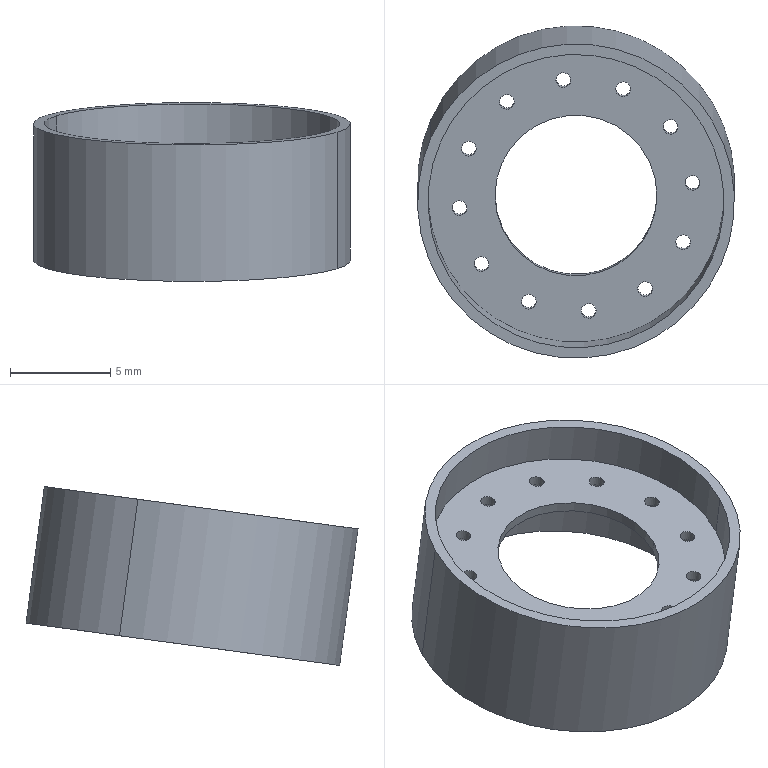Part | SolidWorks | features SplitBody 1 | 1 solid | 36 faces | box 15.84 x 16.618 x 8.937 mm | volume 235.523 mm3 | cylinder 32 | plane 4 | commonest cylinder face diameters 0.739 x24 14.784 x4 8.096 x2 15.84 x2
STEP:
#1=CARTESIAN_POINT('',(537.408,368.019,-344.232));
#2=VERTEX_POINT('',#1);
#3=CARTESIAN_POINT('',(550.937,362.113,-345.028));
#4=VERTEX_POINT('',#3);
#5=CARTESIAN_POINT('',(544.173,365.066,-344.63));
#6=DIRECTION('',(0.,0.1337,-0.991));
#7=DIRECTION('',(0.9151,-0.3995,-0.05388));
#8=AXIS2_PLACEMENT_3D('',#5,#6,#7);
#9=CIRCLE('',#8,7.392);
#10=EDGE_CURVE('',#2,#4,#9,.T.);
#11=ORIENTED_EDGE('',*,*,#10,.T.);
#12=CARTESIAN_POINT('',(550.937,361.546,-340.825));
#13=VERTEX_POINT('',#12);
#14=CARTESIAN_POINT('',(550.937,362.113,-345.028));
#15=DIRECTION('',(0.,-0.1337,0.991));
#16=VECTOR('',#15,1000.);
#17=LINE('',#14,#16);
#18=EDGE_CURVE('',#4,#13,#17,.T.);
#19=ORIENTED_EDGE('',*,*,#18,.T.);
#20=CARTESIAN_POINT('',(537.408,367.452,-340.028));
#21=VERTEX_POINT('',#20);
#22=CARTESIAN_POINT('',(544.173,364.499,-340.427));
#23=DIRECTION('',(0.,0.1337,-0.991));
#24=DIRECTION('',(0.9151,-0.3995,-0.05388));
#25=AXIS2_PLACEMENT_3D('',#22,#23,#24);
#26=CIRCLE('',#25,7.392);
#27=EDGE_CURVE('',#21,#13,#26,.T.);
#28=ORIENTED_EDGE('',*,*,#27,.F.);
#29=CARTESIAN_POINT('',(537.408,368.019,-344.232));
#30=DIRECTION('',(0.,-0.1337,0.991));
#31=VECTOR('',#30,1000.);
#32=LINE('',#29,#31);
#33=EDGE_CURVE('',#2,#21,#32,.T.);
#34=ORIENTED_EDGE('',*,*,#33,.F.);
#35=EDGE_LOOP('',(#11,#19,#28,#34));
#36=FACE_OUTER_BOUND('',#35,.T.);
#37=CARTESIAN_POINT('',(544.173,365.066,-344.63));
#38=DIRECTION('',(0.,-0.1337,0.991));
#39=DIRECTION('',(-0.9151,0.3995,0.05388));
#40=AXIS2_PLACEMENT_3D('',#37,#38,#39);
#41=CYLINDRICAL_SURFACE('',#40,7.392);
#42=ADVANCED_FACE('',(#36),#41,.F.);
#43=CARTESIAN_POINT('',(539.79,360.853,-340.385));
#44=VERTEX_POINT('',#43);
#45=CARTESIAN_POINT('',(539.114,361.149,-340.346));
#46=VERTEX_POINT('',#45);
#47=CARTESIAN_POINT('',(539.452,361.001,-340.366));
#48=DIRECTION('',(0.,-0.1337,0.991));
#49=DIRECTION('',(-0.9151,0.3995,0.05388));
#50=AXIS2_PLACEMENT_3D('',#47,#48,#49);
#51=CIRCLE('',#50,0.3696);
#52=EDGE_CURVE('',#44,#46,#51,.T.);
#53=ORIENTED_EDGE('',*,*,#52,.T.);
#54=CARTESIAN_POINT('',(539.114,361.219,-340.869));
#55=VERTEX_POINT('',#54);
#56=CARTESIAN_POINT('',(539.114,361.219,-340.869));
#57=DIRECTION('',(0.,0.1337,-0.991));
#58=VECTOR('',#57,1000.);
#59=LINE('',#56,#58);
#60=EDGE_CURVE('',#46,#55,#59,.T.);
#61=ORIENTED_EDGE('',*,*,#60,.T.);
#62=CARTESIAN_POINT('',(539.79,360.924,-340.909));
#63=VERTEX_POINT('',#62);
#64=CARTESIAN_POINT('',(539.452,361.072,-340.889));
#65=DIRECTION('',(0.,0.1337,-0.991));
#66=DIRECTION('',(0.9151,-0.3995,-0.05388));
#67=AXIS2_PLACEMENT_3D('',#64,#65,#66);
#68=CIRCLE('',#67,0.3696);
#69=EDGE_CURVE('',#55,#63,#68,.T.);
#70=ORIENTED_EDGE('',*,*,#69,.T.);
#71=CARTESIAN_POINT('',(539.79,360.924,-340.909));
#72=DIRECTION('',(0.,0.1337,-0.991));
#73=VECTOR('',#72,1000.);
#74=LINE('',#71,#73);
#75=EDGE_CURVE('',#44,#63,#74,.T.);
#76=ORIENTED_EDGE('',*,*,#75,.F.);
#77=EDGE_LOOP('',(#53,#61,#70,#76));
#78=FACE_OUTER_BOUND('',#77,.T.);
#79=CARTESIAN_POINT('',(539.452,361.072,-340.889));
#80=DIRECTION('',(0.,0.1337,-0.991));
#81=DIRECTION('',(0.9151,-0.3995,-0.05388));
#82=AXIS2_PLACEMENT_3D('',#79,#80,#81);
#83=CYLINDRICAL_SURFACE('',#82,0.3696);
#84=ADVANCED_FACE('',(#78),#83,.F.);
#85=CARTESIAN_POINT('',(538.693,363.652,-340.008));
#86=VERTEX_POINT('',#85);
#87=CARTESIAN_POINT('',(538.017,363.947,-339.968));
#88=VERTEX_POINT('',#87);
#89=CARTESIAN_POINT('',(538.355,363.799,-339.988));
#90=DIRECTION('',(0.,-0.1337,0.991));
#91=DIRECTION('',(-0.9151,0.3995,0.05388));
#92=AXIS2_PLACEMENT_3D('',#89,#90,#91);
#93=CIRCLE('',#92,0.3696);
#94=EDGE_CURVE('',#86,#88,#93,.T.);
#95=ORIENTED_EDGE('',*,*,#94,.T.);
#96=CARTESIAN_POINT('',(538.017,364.018,-340.492));
#97=VERTEX_POINT('',#96);
#98=CARTESIAN_POINT('',(538.017,364.018,-340.492));
#99=DIRECTION('',(0.,0.1337,-0.991));
#100=VECTOR('',#99,1000.);
#101=LINE('',#98,#100);
#102=EDGE_CURVE('',#88,#97,#101,.T.);
#103=ORIENTED_EDGE('',*,*,#102,.T.);
#104=CARTESIAN_POINT('',(538.693,363.722,-340.531));
#105=VERTEX_POINT('',#104);
#106=CARTESIAN_POINT('',(538.355,363.87,-340.511));
#107=DIRECTION('',(0.,0.1337,-0.991));
#108=DIRECTION('',(0.9151,-0.3995,-0.05388));
#109=AXIS2_PLACEMENT_3D('',#106,#107,#108);
#110=CIRCLE('',#109,0.3696);
#111=EDGE_CURVE('',#97,#105,#110,.T.);
#112=ORIENTED_EDGE('',*,*,#111,.T.);
#113=CARTESIAN_POINT('',(538.693,363.722,-340.531));
#114=DIRECTION('',(0.,0.1337,-0.991));
#115=VECTOR('',#114,1000.);
#116=LINE('',#113,#115);
#117=EDGE_CURVE('',#86,#105,#116,.T.);
#118=ORIENTED_EDGE('',*,*,#117,.F.);
#119=EDGE_LOOP('',(#95,#103,#112,#118));
#120=FACE_OUTER_BOUND('',#119,.T.);
#121=CARTESIAN_POINT('',(538.355,363.87,-340.511));
#122=DIRECTION('',(0.,0.1337,-0.991));
#123=DIRECTION('',(0.9151,-0.3995,-0.05388));
#124=AXIS2_PLACEMENT_3D('',#121,#122,#123);
#125=CYLINDRICAL_SURFACE('',#124,0.3696);
#126=ADVANCED_FACE('',(#120),#125,.F.);
#127=CARTESIAN_POINT('',(539.155,366.619,-339.608));
#128=VERTEX_POINT('',#127);
#129=CARTESIAN_POINT('',(538.479,366.914,-339.568));
#130=VERTEX_POINT('',#129);
#131=CARTESIAN_POINT('',(538.817,366.766,-339.588));
#132=DIRECTION('',(0.,-0.1337,0.991));
#133=DIRECTION('',(-0.9151,0.3995,0.05388));
#134=AXIS2_PLACEMENT_3D('',#131,#132,#133);
#135=CIRCLE('',#134,0.3696);
#136=EDGE_CURVE('',#128,#130,#135,.T.);
#137=ORIENTED_EDGE('',*,*,#136,.T.);
#138=CARTESIAN_POINT('',(538.479,366.985,-340.091));
#139=VERTEX_POINT('',#138);
#140=CARTESIAN_POINT('',(538.479,366.985,-340.091));
#141=DIRECTION('',(0.,0.1337,-0.991));
#142=VECTOR('',#141,1000.);
#143=LINE('',#140,#142);
#144=EDGE_CURVE('',#130,#139,#143,.T.);
#145=ORIENTED_EDGE('',*,*,#144,.T.);
#146=CARTESIAN_POINT('',(539.155,366.689,-340.131));
#147=VERTEX_POINT('',#146);
#148=CARTESIAN_POINT('',(538.817,366.837,-340.111));
#149=DIRECTION('',(0.,0.1337,-0.991));
#150=DIRECTION('',(0.9151,-0.3995,-0.05388));
#151=AXIS2_PLACEMENT_3D('',#148,#149,#150);
#152=CIRCLE('',#151,0.3696);
#153=EDGE_CURVE('',#139,#147,#152,.T.);
#154=ORIENTED_EDGE('',*,*,#153,.T.);
#155=CARTESIAN_POINT('',(539.155,366.689,-340.131));
#156=DIRECTION('',(0.,0.1337,-0.991));
#157=VECTOR('',#156,1000.);
#158=LINE('',#155,#157);
#159=EDGE_CURVE('',#128,#147,#158,.T.);
#160=ORIENTED_EDGE('',*,*,#159,.F.);
#161=EDGE_LOOP('',(#137,#145,#154,#160));
#162=FACE_OUTER_BOUND('',#161,.T.);
#163=CARTESIAN_POINT('',(538.817,366.837,-340.111));
#164=DIRECTION('',(0.,0.1337,-0.991));
#165=DIRECTION('',(0.9151,-0.3995,-0.05388));
#166=AXIS2_PLACEMENT_3D('',#163,#164,#165);
#167=CYLINDRICAL_SURFACE('',#166,0.3696);
#168=ADVANCED_FACE('',(#162),#167,.F.);
#169=CARTESIAN_POINT('',(541.052,368.959,-339.292));
#170=VERTEX_POINT('',#169);
#171=CARTESIAN_POINT('',(540.376,369.254,-339.252));
#172=VERTEX_POINT('',#171);
#173=CARTESIAN_POINT('',(540.714,369.107,-339.272));
#174=DIRECTION('',(0.,-0.1337,0.991));
#175=DIRECTION('',(-0.9151,0.3995,0.05388));
#176=AXIS2_PLACEMENT_3D('',#173,#174,#175);
#177=CIRCLE('',#176,0.3696);
#178=EDGE_CURVE('',#170,#172,#177,.T.);
#179=ORIENTED_EDGE('',*,*,#178,.T.);
#180=CARTESIAN_POINT('',(540.376,369.325,-339.776));
#181=VERTEX_POINT('',#180);
#182=CARTESIAN_POINT('',(540.376,369.325,-339.776));
#183=DIRECTION('',(0.,0.1337,-0.991));
#184=VECTOR('',#183,1000.);
#185=LINE('',#182,#184);
#186=EDGE_CURVE('',#172,#181,#185,.T.);
#187=ORIENTED_EDGE('',*,*,#186,.T.);
#188=CARTESIAN_POINT('',(541.052,369.03,-339.816));
#189=VERTEX_POINT('',#188);
#190=CARTESIAN_POINT('',(540.714,369.177,-339.796));
#191=DIRECTION('',(0.,0.1337,-0.991));
#192=DIRECTION('',(0.9151,-0.3995,-0.05388));
#193=AXIS2_PLACEMENT_3D('',#190,#191,#192);
#194=CIRCLE('',#193,0.3696);
#195=EDGE_CURVE('',#181,#189,#194,.T.);
#196=ORIENTED_EDGE('',*,*,#195,.T.);
#197=CARTESIAN_POINT('',(541.052,369.03,-339.816));
#198=DIRECTION('',(0.,0.1337,-0.991));
#199=VECTOR('',#198,1000.);
#200=LINE('',#197,#199);
#201=EDGE_CURVE('',#170,#189,#200,.T.);
#202=ORIENTED_EDGE('',*,*,#201,.F.);
#203=EDGE_LOOP('',(#179,#187,#196,#202));
#204=FACE_OUTER_BOUND('',#203,.T.);
#205=CARTESIAN_POINT('',(540.714,369.177,-339.796));
#206=DIRECTION('',(0.,0.1337,-0.991));
#207=DIRECTION('',(0.9151,-0.3995,-0.05388));
#208=AXIS2_PLACEMENT_3D('',#205,#206,#207);
#209=CYLINDRICAL_SURFACE('',#208,0.3696);
#210=ADVANCED_FACE('',(#204),#209,.F.);
#211=CARTESIAN_POINT('',(543.876,370.046,-339.146));
#212=VERTEX_POINT('',#211);
#213=CARTESIAN_POINT('',(543.2,370.341,-339.106));
#214=VERTEX_POINT('',#213);
#215=CARTESIAN_POINT('',(543.538,370.194,-339.126));
#216=DIRECTION('',(0.,-0.1337,0.991));
#217=DIRECTION('',(-0.9151,0.3995,0.05388));
#218=AXIS2_PLACEMENT_3D('',#215,#216,#217);
#219=CIRCLE('',#218,0.3696);
#220=EDGE_CURVE('',#212,#214,#219,.T.);
#221=ORIENTED_EDGE('',*,*,#220,.T.);
#222=CARTESIAN_POINT('',(543.2,370.412,-339.629));
#223=VERTEX_POINT('',#222);
#224=CARTESIAN_POINT('',(543.2,370.412,-339.629));
#225=DIRECTION('',(0.,0.1337,-0.991));
#226=VECTOR('',#225,1000.);
#227=LINE('',#224,#226);
#228=EDGE_CURVE('',#214,#223,#227,.T.);
#229=ORIENTED_EDGE('',*,*,#228,.T.);
#230=CARTESIAN_POINT('',(543.876,370.117,-339.669));
#231=VERTEX_POINT('',#230);
#232=CARTESIAN_POINT('',(543.538,370.264,-339.649));
#233=DIRECTION('',(0.,0.1337,-0.991));
#234=DIRECTION('',(0.9151,-0.3995,-0.05388));
#235=AXIS2_PLACEMENT_3D('',#232,#233,#234);
#236=CIRCLE('',#235,0.3696);
#237=EDGE_CURVE('',#223,#231,#236,.T.);
#238=ORIENTED_EDGE('',*,*,#237,.T.);
#239=CARTESIAN_POINT('',(543.876,370.117,-339.669));
#240=DIRECTION('',(0.,0.1337,-0.991));
#241=VECTOR('',#240,1000.);
#242=LINE('',#239,#241);
#243=EDGE_CURVE('',#212,#231,#242,.T.);
#244=ORIENTED_EDGE('',*,*,#243,.F.);
#245=EDGE_LOOP('',(#221,#229,#238,#244));
#246=FACE_OUTER_BOUND('',#245,.T.);
#247=CARTESIAN_POINT('',(543.538,370.264,-339.649));
#248=DIRECTION('',(0.,0.1337,-0.991));
#249=DIRECTION('',(0.9151,-0.3995,-0.05388));
#250=AXIS2_PLACEMENT_3D('',#247,#248,#249);
#251=CYLINDRICAL_SURFACE('',#250,0.3696);
#252=ADVANCED_FACE('',(#246),#251,.F.);
#253=CARTESIAN_POINT('',(546.87,369.588,-339.207));
#254=VERTEX_POINT('',#253);
#255=CARTESIAN_POINT('',(546.193,369.883,-339.168));
#256=VERTEX_POINT('',#255);
#257=CARTESIAN_POINT('',(546.532,369.736,-339.188));
#258=DIRECTION('',(0.,-0.1337,0.991));
#259=DIRECTION('',(-0.9151,0.3995,0.05388));
#260=AXIS2_PLACEMENT_3D('',#257,#258,#259);
#261=CIRCLE('',#260,0.3696);
#262=EDGE_CURVE('',#254,#256,#261,.T.);
#263=ORIENTED_EDGE('',*,*,#262,.T.);
#264=CARTESIAN_POINT('',(546.193,369.954,-339.691));
#265=VERTEX_POINT('',#264);
#266=CARTESIAN_POINT('',(546.193,369.954,-339.691));
#267=DIRECTION('',(0.,0.1337,-0.991));
#268=VECTOR('',#267,1000.);
#269=LINE('',#266,#268);
#270=EDGE_CURVE('',#256,#265,#269,.T.);
#271=ORIENTED_EDGE('',*,*,#270,.T.);
#272=CARTESIAN_POINT('',(546.87,369.659,-339.731));
#273=VERTEX_POINT('',#272);
#274=CARTESIAN_POINT('',(546.532,369.806,-339.711));
#275=DIRECTION('',(0.,0.1337,-0.991));
#276=DIRECTION('',(0.9151,-0.3995,-0.05388));
#277=AXIS2_PLACEMENT_3D('',#274,#275,#276);
#278=CIRCLE('',#277,0.3696);
#279=EDGE_CURVE('',#265,#273,#278,.T.);
#280=ORIENTED_EDGE('',*,*,#279,.T.);
#281=CARTESIAN_POINT('',(546.87,369.659,-339.731));
#282=DIRECTION('',(0.,0.1337,-0.991));
#283=VECTOR('',#282,1000.);
#284=LINE('',#281,#283);
#285=EDGE_CURVE('',#254,#273,#284,.T.);
#286=ORIENTED_EDGE('',*,*,#285,.F.);
#287=EDGE_LOOP('',(#263,#271,#280,#286));
#288=FACE_OUTER_BOUND('',#287,.T.);
#289=CARTESIAN_POINT('',(546.532,369.806,-339.711));
#290=DIRECTION('',(0.,0.1337,-0.991));
#291=DIRECTION('',(0.9151,-0.3995,-0.05388));
#292=AXIS2_PLACEMENT_3D('',#289,#290,#291);
#293=CYLINDRICAL_SURFACE('',#292,0.3696);
#294=ADVANCED_FACE('',(#288),#293,.F.);
#295=CARTESIAN_POINT('',(549.232,367.708,-339.461));
#296=VERTEX_POINT('',#295);
#297=CARTESIAN_POINT('',(548.555,368.003,-339.421));
#298=VERTEX_POINT('',#297);
#299=CARTESIAN_POINT('',(548.893,367.856,-339.441));
#300=DIRECTION('',(0.,-0.1337,0.991));
#301=DIRECTION('',(-0.9151,0.3995,0.05388));
#302=AXIS2_PLACEMENT_3D('',#299,#300,#301);
#303=CIRCLE('',#302,0.3696);
#304=EDGE_CURVE('',#296,#298,#303,.T.);
#305=ORIENTED_EDGE('',*,*,#304,.T.);
#306=CARTESIAN_POINT('',(548.555,368.074,-339.944));
#307=VERTEX_POINT('',#306);
#308=CARTESIAN_POINT('',(548.555,368.074,-339.944));
#309=DIRECTION('',(0.,0.1337,-0.991));
#310=VECTOR('',#309,1000.);
#311=LINE('',#308,#310);
#312=EDGE_CURVE('',#298,#307,#311,.T.);
#313=ORIENTED_EDGE('',*,*,#312,.T.);
#314=CARTESIAN_POINT('',(549.232,367.779,-339.984));
#315=VERTEX_POINT('',#314);
#316=CARTESIAN_POINT('',(548.893,367.926,-339.964));
#317=DIRECTION('',(0.,0.1337,-0.991));
#318=DIRECTION('',(0.9151,-0.3995,-0.05388));
#319=AXIS2_PLACEMENT_3D('',#316,#317,#318);
#320=CIRCLE('',#319,0.3696);
#321=EDGE_CURVE('',#307,#315,#320,.T.);
#322=ORIENTED_EDGE('',*,*,#321,.T.);
#323=CARTESIAN_POINT('',(549.232,367.779,-339.984));
#324=DIRECTION('',(0.,0.1337,-0.991));
#325=VECTOR('',#324,1000.);
#326=LINE('',#323,#325);
#327=EDGE_CURVE('',#296,#315,#326,.T.);
#328=ORIENTED_EDGE('',*,*,#327,.F.);
#329=EDGE_LOOP('',(#305,#313,#322,#328));
#330=FACE_OUTER_BOUND('',#329,.T.);
#331=CARTESIAN_POINT('',(548.893,367.926,-339.964));
#332=DIRECTION('',(0.,0.1337,-0.991));
#333=DIRECTION('',(0.9151,-0.3995,-0.05388));
#334=AXIS2_PLACEMENT_3D('',#331,#332,#333);
#335=CYLINDRICAL_SURFACE('',#334,0.3696);
#336=ADVANCED_FACE('',(#330),#335,.F.);
#337=CARTESIAN_POINT('',(550.328,364.91,-339.838));
#338=VERTEX_POINT('',#337);
#339=CARTESIAN_POINT('',(549.652,365.205,-339.799));
#340=VERTEX_POINT('',#339);
#341=CARTESIAN_POINT('',(549.99,365.057,-339.818));
#342=DIRECTION('',(0.,-0.1337,0.991));
#343=DIRECTION('',(-0.9151,0.3995,0.05388));
#344=AXIS2_PLACEMENT_3D('',#341,#342,#343);
#345=CIRCLE('',#344,0.3696);
#346=EDGE_CURVE('',#338,#340,#345,.T.);
#347=ORIENTED_EDGE('',*,*,#346,.T.);
#348=CARTESIAN_POINT('',(549.652,365.276,-340.322));
#349=VERTEX_POINT('',#348);
#350=CARTESIAN_POINT('',(549.652,365.276,-340.322));
#351=DIRECTION('',(0.,0.1337,-0.991));
#352=VECTOR('',#351,1000.);
#353=LINE('',#350,#352);
#354=EDGE_CURVE('',#340,#349,#353,.T.);
#355=ORIENTED_EDGE('',*,*,#354,.T.);
#356=CARTESIAN_POINT('',(550.328,364.98,-340.362));
#357=VERTEX_POINT('',#356);
#358=CARTESIAN_POINT('',(549.99,365.128,-340.342));
#359=DIRECTION('',(0.,0.1337,-0.991));
#360=DIRECTION('',(0.9151,-0.3995,-0.05388));
#361=AXIS2_PLACEMENT_3D('',#358,#359,#360);
#362=CIRCLE('',#361,0.3696);
#363=EDGE_CURVE('',#349,#357,#362,.T.);
#364=ORIENTED_EDGE('',*,*,#363,.T.);
#365=CARTESIAN_POINT('',(550.328,364.98,-340.362));
#366=DIRECTION('',(0.,0.1337,-0.991));
#367=VECTOR('',#366,1000.);
#368=LINE('',#365,#367);
#369=EDGE_CURVE('',#338,#357,#368,.T.);
#370=ORIENTED_EDGE('',*,*,#369,.F.);
#371=EDGE_LOOP('',(#347,#355,#364,#370));
#372=FACE_OUTER_BOUND('',#371,.T.);
#373=CARTESIAN_POINT('',(549.99,365.128,-340.342));
#374=DIRECTION('',(0.,0.1337,-0.991));
#375=DIRECTION('',(0.9151,-0.3995,-0.05388));
#376=AXIS2_PLACEMENT_3D('',#373,#374,#375);
#377=CYLINDRICAL_SURFACE('',#376,0.3696);
#378=ADVANCED_FACE('',(#372),#377,.F.);
#379=CARTESIAN_POINT('',(549.866,361.943,-340.239));
#380=VERTEX_POINT('',#379);
#381=CARTESIAN_POINT('',(549.19,362.238,-340.199));
#382=VERTEX_POINT('',#381);
#383=CARTESIAN_POINT('',(549.528,362.091,-340.219));
#384=DIRECTION('',(0.,-0.1337,0.991));
#385=DIRECTION('',(-0.9151,0.3995,0.05388));
#386=AXIS2_PLACEMENT_3D('',#383,#384,#385);
#387=CIRCLE('',#386,0.3696);
#388=EDGE_CURVE('',#380,#382,#387,.T.);
#389=ORIENTED_EDGE('',*,*,#388,.T.);
#390=CARTESIAN_POINT('',(549.19,362.309,-340.722));
#391=VERTEX_POINT('',#390);
#392=CARTESIAN_POINT('',(549.19,362.309,-340.722));
#393=DIRECTION('',(0.,0.1337,-0.991));
#394=VECTOR('',#393,1000.);
#395=LINE('',#392,#394);
#396=EDGE_CURVE('',#382,#391,#395,.T.);
#397=ORIENTED_EDGE('',*,*,#396,.T.);
#398=CARTESIAN_POINT('',(549.866,362.013,-340.762));
#399=VERTEX_POINT('',#398);
#400=CARTESIAN_POINT('',(549.528,362.161,-340.742));
#401=DIRECTION('',(0.,0.1337,-0.991));
#402=DIRECTION('',(0.9151,-0.3995,-0.05388));
#403=AXIS2_PLACEMENT_3D('',#400,#401,#402);
#404=CIRCLE('',#403,0.3696);
#405=EDGE_CURVE('',#391,#399,#404,.T.);
#406=ORIENTED_EDGE('',*,*,#405,.T.);
#407=CARTESIAN_POINT('',(549.866,362.013,-340.762));
#408=DIRECTION('',(0.,0.1337,-0.991));
#409=VECTOR('',#408,1000.);
#410=LINE('',#407,#409);
#411=EDGE_CURVE('',#380,#399,#410,.T.);
#412=ORIENTED_EDGE('',*,*,#411,.F.);
#413=EDGE_LOOP('',(#389,#397,#406,#412));
#414=FACE_OUTER_BOUND('',#413,.T.);
#415=CARTESIAN_POINT('',(549.528,362.161,-340.742));
#416=DIRECTION('',(0.,0.1337,-0.991));
#417=DIRECTION('',(0.9151,-0.3995,-0.05388));
#418=AXIS2_PLACEMENT_3D('',#415,#416,#417);
#419=CYLINDRICAL_SURFACE('',#418,0.3696);
#420=ADVANCED_FACE('',(#414),#419,.F.);
#421=CARTESIAN_POINT('',(547.969,359.602,-340.554));
#422=VERTEX_POINT('',#421);
#423=CARTESIAN_POINT('',(547.293,359.898,-340.514));
#424=VERTEX_POINT('',#423);
#425=CARTESIAN_POINT('',(547.631,359.75,-340.534));
#426=DIRECTION('',(0.,-0.1337,0.991));
#427=DIRECTION('',(-0.9151,0.3995,0.05388));
#428=AXIS2_PLACEMENT_3D('',#425,#426,#427);
#429=CIRCLE('',#428,0.3696);
#430=EDGE_CURVE('',#422,#424,#429,.T.);
#431=ORIENTED_EDGE('',*,*,#430,.T.);
#432=CARTESIAN_POINT('',(547.293,359.968,-341.038));
#433=VERTEX_POINT('',#432);
#434=CARTESIAN_POINT('',(547.293,359.968,-341.038));
#435=DIRECTION('',(0.,0.1337,-0.991));
#436=VECTOR('',#435,1000.);
#437=LINE('',#434,#436);
#438=EDGE_CURVE('',#424,#433,#437,.T.);
#439=ORIENTED_EDGE('',*,*,#438,.T.);
#440=CARTESIAN_POINT('',(547.969,359.673,-341.077));
#441=VERTEX_POINT('',#440);
#442=CARTESIAN_POINT('',(547.631,359.821,-341.058));
#443=DIRECTION('',(0.,0.1337,-0.991));
#444=DIRECTION('',(0.9151,-0.3995,-0.05388));
#445=AXIS2_PLACEMENT_3D('',#442,#443,#444);
#446=CIRCLE('',#445,0.3696);
#447=EDGE_CURVE('',#433,#441,#446,.T.);
#448=ORIENTED_EDGE('',*,*,#447,.T.);
#449=CARTESIAN_POINT('',(547.969,359.673,-341.077));
#450=DIRECTION('',(0.,0.1337,-0.991));
#451=VECTOR('',#450,1000.);
#452=LINE('',#449,#451);
#453=EDGE_CURVE('',#422,#441,#452,.T.);
#454=ORIENTED_EDGE('',*,*,#453,.F.);
#455=EDGE_LOOP('',(#431,#439,#448,#454));
#456=FACE_OUTER_BOUND('',#455,.T.);
#457=CARTESIAN_POINT('',(547.631,359.821,-341.058));
#458=DIRECTION('',(0.,0.1337,-0.991));
#459=DIRECTION('',(0.9151,-0.3995,-0.05388));
#460=AXIS2_PLACEMENT_3D('',#457,#458,#459);
#461=CYLINDRICAL_SURFACE('',#460,0.3696);
#462=ADVANCED_FACE('',(#456),#461,.F.);
#463=CARTESIAN_POINT('',(545.146,358.515,-340.701));
#464=VERTEX_POINT('',#463);
#465=CARTESIAN_POINT('',(544.469,358.811,-340.661));
#466=VERTEX_POINT('',#465);
#467=CARTESIAN_POINT('',(544.807,358.663,-340.681));
#468=DIRECTION('',(0.,-0.1337,0.991));
#469=DIRECTION('',(-0.9151,0.3995,0.05388));
#470=AXIS2_PLACEMENT_3D('',#467,#468,#469);
#471=CIRCLE('',#470,0.3696);
#472=EDGE_CURVE('',#464,#466,#471,.T.);
#473=ORIENTED_EDGE('',*,*,#472,.T.);
#474=CARTESIAN_POINT('',(544.469,358.881,-341.184));
#475=VERTEX_POINT('',#474);
#476=CARTESIAN_POINT('',(544.469,358.881,-341.184));
#477=DIRECTION('',(0.,0.1337,-0.991));
#478=VECTOR('',#477,1000.);
#479=LINE('',#476,#478);
#480=EDGE_CURVE('',#466,#475,#479,.T.);
#481=ORIENTED_EDGE('',*,*,#480,.T.);
#482=CARTESIAN_POINT('',(545.146,358.586,-341.224));
#483=VERTEX_POINT('',#482);
#484=CARTESIAN_POINT('',(544.807,358.734,-341.204));
#485=DIRECTION('',(0.,0.1337,-0.991));
#486=DIRECTION('',(0.9151,-0.3995,-0.05388));
#487=AXIS2_PLACEMENT_3D('',#484,#485,#486);
#488=CIRCLE('',#487,0.3696);
#489=EDGE_CURVE('',#475,#483,#488,.T.);
#490=ORIENTED_EDGE('',*,*,#489,.T.);
#491=CARTESIAN_POINT('',(545.146,358.586,-341.224));
#492=DIRECTION('',(0.,0.1337,-0.991));
#493=VECTOR('',#492,1000.);
#494=LINE('',#491,#493);
#495=EDGE_CURVE('',#464,#483,#494,.T.);
#496=ORIENTED_EDGE('',*,*,#495,.F.);
#497=EDGE_LOOP('',(#473,#481,#490,#496));
#498=FACE_OUTER_BOUND('',#497,.T.);
#499=CARTESIAN_POINT('',(544.807,358.734,-341.204));
#500=DIRECTION('',(0.,0.1337,-0.991));
#501=DIRECTION('',(0.9151,-0.3995,-0.05388));
#502=AXIS2_PLACEMENT_3D('',#499,#500,#501);
#503=CYLINDRICAL_SURFACE('',#502,0.3696);
#504=ADVANCED_FACE('',(#498),#503,.F.);
#505=CARTESIAN_POINT('',(542.152,358.973,-340.639));
#506=VERTEX_POINT('',#505);
#507=CARTESIAN_POINT('',(541.475,359.269,-340.599));
#508=VERTEX_POINT('',#507);
#509=CARTESIAN_POINT('',(541.813,359.121,-340.619));
#510=DIRECTION('',(0.,-0.1337,0.991));
#511=DIRECTION('',(-0.9151,0.3995,0.05388));
#512=AXIS2_PLACEMENT_3D('',#509,#510,#511);
#513=CIRCLE('',#512,0.3696);
#514=EDGE_CURVE('',#506,#508,#513,.T.);
#515=ORIENTED_EDGE('',*,*,#514,.T.);
#516=CARTESIAN_POINT('',(541.475,359.339,-341.122));
#517=VERTEX_POINT('',#516);
#518=CARTESIAN_POINT('',(541.475,359.339,-341.122));
#519=DIRECTION('',(0.,0.1337,-0.991));
#520=VECTOR('',#519,1000.);
#521=LINE('',#518,#520);
#522=EDGE_CURVE('',#508,#517,#521,.T.);
#523=ORIENTED_EDGE('',*,*,#522,.T.);
#524=CARTESIAN_POINT('',(542.152,359.044,-341.162));
#525=VERTEX_POINT('',#524);
#526=CARTESIAN_POINT('',(541.813,359.192,-341.142));
#527=DIRECTION('',(0.,0.1337,-0.991));
#528=DIRECTION('',(0.9151,-0.3995,-0.05388));
#529=AXIS2_PLACEMENT_3D('',#526,#527,#528);
#530=CIRCLE('',#529,0.3696);
#531=EDGE_CURVE('',#517,#525,#530,.T.);
#532=ORIENTED_EDGE('',*,*,#531,.T.);
#533=CARTESIAN_POINT('',(542.152,359.044,-341.162));
#534=DIRECTION('',(0.,0.1337,-0.991));
#535=VECTOR('',#534,1000.);
#536=LINE('',#533,#535);
#537=EDGE_CURVE('',#506,#525,#536,.T.);
#538=ORIENTED_EDGE('',*,*,#537,.F.);
#539=EDGE_LOOP('',(#515,#523,#532,#538));
#540=FACE_OUTER_BOUND('',#539,.T.);
#541=CARTESIAN_POINT('',(541.813,359.192,-341.142));
#542=DIRECTION('',(0.,0.1337,-0.991));
#543=DIRECTION('',(0.9151,-0.3995,-0.05388));
#544=AXIS2_PLACEMENT_3D('',#541,#542,#543);
#545=CYLINDRICAL_SURFACE('',#544,0.3696);
#546=ADVANCED_FACE('',(#540),#545,.F.);
#547=CARTESIAN_POINT('',(547.877,362.882,-340.645));
#548=VERTEX_POINT('',#547);
#549=CARTESIAN_POINT('',(540.468,366.116,-340.208));
#550=VERTEX_POINT('',#549);
#551=CARTESIAN_POINT('',(544.173,364.499,-340.427));
#552=DIRECTION('',(0.,-0.1337,0.991));
#553=DIRECTION('',(-0.9151,0.3995,0.05388));
#554=AXIS2_PLACEMENT_3D('',#551,#552,#553);
#555=CIRCLE('',#554,4.048);
#556=EDGE_CURVE('',#548,#550,#555,.T.);
#557=ORIENTED_EDGE('',*,*,#556,.F.);
#558=CARTESIAN_POINT('',(547.877,362.811,-340.121));
#559=VERTEX_POINT('',#558);
#560=CARTESIAN_POINT('',(547.877,362.882,-340.645));
#561=DIRECTION('',(0.,-0.1337,0.991));
#562=VECTOR('',#561,1000.);
#563=LINE('',#560,#562);
#564=EDGE_CURVE('',#548,#559,#563,.T.);
#565=ORIENTED_EDGE('',*,*,#564,.T.);
#566=CARTESIAN_POINT('',(540.468,366.046,-339.685));
#567=VERTEX_POINT('',#566);
#568=CARTESIAN_POINT('',(544.173,364.428,-339.903));
#569=DIRECTION('',(0.,-0.1337,0.991));
#570=DIRECTION('',(-0.9151,0.3995,0.05388));
#571=AXIS2_PLACEMENT_3D('',#568,#569,#570);
#572=CIRCLE('',#571,4.048);
#573=EDGE_CURVE('',#559,#567,#572,.T.);
#574=ORIENTED_EDGE('',*,*,#573,.T.);
#575=CARTESIAN_POINT('',(540.468,366.116,-340.208));
#576=DIRECTION('',(0.,-0.1337,0.991));
#577=VECTOR('',#576,1000.);
#578=LINE('',#575,#577);
#579=EDGE_CURVE('',#550,#567,#578,.T.);
#580=ORIENTED_EDGE('',*,*,#579,.F.);
#581=EDGE_LOOP('',(#557,#565,#574,#580));
#582=FACE_OUTER_BOUND('',#581,.T.);
#583=CARTESIAN_POINT('',(544.173,364.499,-340.427));
#584=DIRECTION('',(0.,-0.1337,0.991));
#585=DIRECTION('',(-0.9151,0.3995,0.05388));
#586=AXIS2_PLACEMENT_3D('',#583,#584,#585);
#587=CYLINDRICAL_SURFACE('',#586,4.048);
#588=ADVANCED_FACE('',(#582),#587,.F.);
#589=CARTESIAN_POINT('',(537.408,367.099,-337.412));
#590=VERTEX_POINT('',#589);
#591=CARTESIAN_POINT('',(550.937,361.193,-338.209));
#592=VERTEX_POINT('',#591);
#593=CARTESIAN_POINT('',(544.173,364.146,-337.81));
#594=DIRECTION('',(0.,0.1337,-0.991));
#595=DIRECTION('',(0.9151,-0.3995,-0.05388));
#596=AXIS2_PLACEMENT_3D('',#593,#594,#595);
#597=CIRCLE('',#596,7.392);
#598=EDGE_CURVE('',#590,#592,#597,.T.);
#599=ORIENTED_EDGE('',*,*,#598,.F.);
#600=CARTESIAN_POINT('',(537.408,367.382,-339.505));
#601=VERTEX_POINT('',#600);
#602=CARTESIAN_POINT('',(537.408,367.379,-339.488));
#603=DIRECTION('',(0.,0.1337,-0.991));
#604=VECTOR('',#603,1000.);
#605=LINE('',#602,#604);
#606=EDGE_CURVE('',#590,#601,#605,.T.);
#607=ORIENTED_EDGE('',*,*,#606,.T.);
#608=CARTESIAN_POINT('',(550.937,361.475,-340.302));
#609=VERTEX_POINT('',#608);
#610=CARTESIAN_POINT('',(544.173,364.428,-339.903));
#611=DIRECTION('',(0.,-0.1337,0.991));
#612=DIRECTION('',(-0.9151,0.3995,0.05388));
#613=AXIS2_PLACEMENT_3D('',#610,#611,#612);
#614=CIRCLE('',#613,7.392);
#615=EDGE_CURVE('',#609,#601,#614,.T.);
#616=ORIENTED_EDGE('',*,*,#615,.F.);
#617=CARTESIAN_POINT('',(550.937,361.473,-340.284));
#618=DIRECTION('',(0.,0.1337,-0.991));
#619=VECTOR('',#618,1000.);
#620=LINE('',#617,#619);
#621=EDGE_CURVE('',#592,#609,#620,.T.);
#622=ORIENTED_EDGE('',*,*,#621,.F.);
#623=EDGE_LOOP('',(#599,#607,#616,#622));
#624=FACE_OUTER_BOUND('',#623,.T.);
#625=CARTESIAN_POINT('',(544.173,364.426,-339.886));
#626=DIRECTION('',(0.,0.1337,-0.991));
#627=DIRECTION('',(0.9151,-0.3995,-0.05388));
#628=AXIS2_PLACEMENT_3D('',#625,#626,#627);
#629=CYLINDRICAL_SURFACE('',#628,7.392);
#630=ADVANCED_FACE('',(#624),#629,.F.);
#631=CARTESIAN_POINT('',(551.421,360.982,-338.237));
#632=VERTEX_POINT('',#631);
#633=CARTESIAN_POINT('',(536.925,367.31,-337.384));
#634=VERTEX_POINT('',#633);
#635=CARTESIAN_POINT('',(544.173,364.146,-337.81));
#636=DIRECTION('',(0.,0.1337,-0.991));
#637=DIRECTION('',(-0.4031,-0.9069,-0.1223));
#638=AXIS2_PLACEMENT_3D('',#635,#636,#637);
#639=CIRCLE('',#638,7.92);
#640=EDGE_CURVE('',#632,#634,#639,.T.);
#641=ORIENTED_EDGE('',*,*,#640,.T.);
#642=CARTESIAN_POINT('',(536.925,368.23,-344.203));
#643=VERTEX_POINT('',#642);
#644=CARTESIAN_POINT('',(536.925,367.59,-339.459));
#645=DIRECTION('',(0.,0.1337,-0.991));
#646=VECTOR('',#645,1000.);
#647=LINE('',#644,#646);
#648=EDGE_CURVE('',#634,#643,#647,.T.);
#649=ORIENTED_EDGE('',*,*,#648,.T.);
#650=CARTESIAN_POINT('',(551.421,361.902,-345.057));
#651=VERTEX_POINT('',#650);
#652=CARTESIAN_POINT('',(544.173,365.066,-344.63));
#653=DIRECTION('',(0.,0.1337,-0.991));
#654=DIRECTION('',(-0.4031,-0.9069,-0.1223));
#655=AXIS2_PLACEMENT_3D('',#652,#653,#654);
#656=CIRCLE('',#655,7.92);
#657=EDGE_CURVE('',#651,#643,#656,.T.);
#658=ORIENTED_EDGE('',*,*,#657,.F.);
#659=CARTESIAN_POINT('',(551.421,361.262,-340.313));
#660=DIRECTION('',(0.,0.1337,-0.991));
#661=VECTOR('',#660,1000.);
#662=LINE('',#659,#661);
#663=EDGE_CURVE('',#632,#651,#662,.T.);
#664=ORIENTED_EDGE('',*,*,#663,.F.);
#665=EDGE_LOOP('',(#641,#649,#658,#664));
#666=FACE_OUTER_BOUND('',#665,.T.);
#667=CARTESIAN_POINT('',(544.173,364.426,-339.886));
#668=DIRECTION('',(0.,0.1337,-0.991));
#669=DIRECTION('',(0.9151,-0.3995,-0.05388));
#670=AXIS2_PLACEMENT_3D('',#667,#668,#669);
#671=CYLINDRICAL_SURFACE('',#670,7.92);
#672=ADVANCED_FACE('',(#666),#671,.T.);
#673=CARTESIAN_POINT('',(539.452,361.072,-340.889));
#674=DIRECTION('',(0.,0.1337,-0.991));
#675=DIRECTION('',(0.9151,-0.3995,-0.05388));
#676=AXIS2_PLACEMENT_3D('',#673,#674,#675);
#677=CIRCLE('',#676,0.3696);
#678=EDGE_CURVE('',#63,#55,#677,.T.);
#679=ORIENTED_EDGE('',*,*,#678,.F.);
#680=ORIENTED_EDGE('',*,*,#69,.F.);
#681=EDGE_LOOP('',(#679,#680));
#682=FACE_BOUND('',#681,.T.);
#683=CARTESIAN_POINT('',(546.532,369.806,-339.711));
#684=DIRECTION('',(0.,0.1337,-0.991));
#685=DIRECTION('',(0.9151,-0.3995,-0.05388));
#686=AXIS2_PLACEMENT_3D('',#683,#684,#685);
#687=CIRCLE('',#686,0.3696);
#688=EDGE_CURVE('',#273,#265,#687,.T.);
#689=ORIENTED_EDGE('',*,*,#688,.F.);
#690=ORIENTED_EDGE('',*,*,#279,.F.);
#691=EDGE_LOOP('',(#689,#690));
#692=FACE_BOUND('',#691,.T.);
#693=CARTESIAN_POINT('',(544.173,364.499,-340.427));
#694=DIRECTION('',(0.,-0.1337,0.991));
#695=DIRECTION('',(-0.9151,0.3995,0.05388));
#696=AXIS2_PLACEMENT_3D('',#693,#694,#695);
#697=CIRCLE('',#696,4.048);
#698=EDGE_CURVE('',#550,#548,#697,.T.);
#699=ORIENTED_EDGE('',*,*,#698,.T.);
#700=ORIENTED_EDGE('',*,*,#556,.T.);
#701=EDGE_LOOP('',(#699,#700));
#702=FACE_BOUND('',#701,.T.);
#703=CARTESIAN_POINT('',(541.813,359.192,-341.142));
#704=DIRECTION('',(0.,0.1337,-0.991));
#705=DIRECTION('',(0.9151,-0.3995,-0.05388));
#706=AXIS2_PLACEMENT_3D('',#703,#704,#705);
#707=CIRCLE('',#706,0.3696);
#708=EDGE_CURVE('',#525,#517,#707,.T.);
#709=ORIENTED_EDGE('',*,*,#708,.F.);
#710=ORIENTED_EDGE('',*,*,#531,.F.);
#711=EDGE_LOOP('',(#709,#710));
#712=FACE_BOUND('',#711,.T.);
#713=CARTESIAN_POINT('',(544.807,358.734,-341.204));
#714=DIRECTION('',(0.,0.1337,-0.991));
#715=DIRECTION('',(0.9151,-0.3995,-0.05388));
#716=AXIS2_PLACEMENT_3D('',#713,#714,#715);
#717=CIRCLE('',#716,0.3696);
#718=EDGE_CURVE('',#483,#475,#717,.T.);
#719=ORIENTED_EDGE('',*,*,#718,.F.);
#720=ORIENTED_EDGE('',*,*,#489,.F.);
#721=EDGE_LOOP('',(#719,#720));
#722=FACE_BOUND('',#721,.T.);
#723=CARTESIAN_POINT('',(547.631,359.821,-341.058));
#724=DIRECTION('',(0.,0.1337,-0.991));
#725=DIRECTION('',(0.9151,-0.3995,-0.05388));
#726=AXIS2_PLACEMENT_3D('',#723,#724,#725);
#727=CIRCLE('',#726,0.3696);
#728=EDGE_CURVE('',#441,#433,#727,.T.);
#729=ORIENTED_EDGE('',*,*,#728,.F.);
#730=ORIENTED_EDGE('',*,*,#447,.F.);
#731=EDGE_LOOP('',(#729,#730));
#732=FACE_BOUND('',#731,.T.);
#733=CARTESIAN_POINT('',(549.528,362.161,-340.742));
#734=DIRECTION('',(0.,0.1337,-0.991));
#735=DIRECTION('',(0.9151,-0.3995,-0.05388));
#736=AXIS2_PLACEMENT_3D('',#733,#734,#735);
#737=CIRCLE('',#736,0.3696);
#738=EDGE_CURVE('',#399,#391,#737,.T.);
#739=ORIENTED_EDGE('',*,*,#738,.F.);
#740=ORIENTED_EDGE('',*,*,#405,.F.);
#741=EDGE_LOOP('',(#739,#740));
#742=FACE_BOUND('',#741,.T.);
#743=CARTESIAN_POINT('',(549.99,365.128,-340.342));
#744=DIRECTION('',(0.,0.1337,-0.991));
#745=DIRECTION('',(0.9151,-0.3995,-0.05388));
#746=AXIS2_PLACEMENT_3D('',#743,#744,#745);
#747=CIRCLE('',#746,0.3696);
#748=EDGE_CURVE('',#357,#349,#747,.T.);
#749=ORIENTED_EDGE('',*,*,#748,.F.);
#750=ORIENTED_EDGE('',*,*,#363,.F.);
#751=EDGE_LOOP('',(#749,#750));
#752=FACE_BOUND('',#751,.T.);
#753=CARTESIAN_POINT('',(548.893,367.926,-339.964));
#754=DIRECTION('',(0.,0.1337,-0.991));
#755=DIRECTION('',(0.9151,-0.3995,-0.05388));
#756=AXIS2_PLACEMENT_3D('',#753,#754,#755);
#757=CIRCLE('',#756,0.3696);
#758=EDGE_CURVE('',#315,#307,#757,.T.);
#759=ORIENTED_EDGE('',*,*,#758,.F.);
#760=ORIENTED_EDGE('',*,*,#321,.F.);
#761=EDGE_LOOP('',(#759,#760));
#762=FACE_BOUND('',#761,.T.);
#763=CARTESIAN_POINT('',(543.538,370.264,-339.649));
#764=DIRECTION('',(0.,0.1337,-0.991));
#765=DIRECTION('',(0.9151,-0.3995,-0.05388));
#766=AXIS2_PLACEMENT_3D('',#763,#764,#765);
#767=CIRCLE('',#766,0.3696);
#768=EDGE_CURVE('',#231,#223,#767,.T.);
#769=ORIENTED_EDGE('',*,*,#768,.F.);
#770=ORIENTED_EDGE('',*,*,#237,.F.);
#771=EDGE_LOOP('',(#769,#770));
#772=FACE_BOUND('',#771,.T.);
#773=CARTESIAN_POINT('',(540.714,369.177,-339.796));
#774=DIRECTION('',(0.,0.1337,-0.991));
#775=DIRECTION('',(0.9151,-0.3995,-0.05388));
#776=AXIS2_PLACEMENT_3D('',#773,#774,#775);
#777=CIRCLE('',#776,0.3696);
#778=EDGE_CURVE('',#189,#181,#777,.T.);
#779=ORIENTED_EDGE('',*,*,#778,.F.);
#780=ORIENTED_EDGE('',*,*,#195,.F.);
#781=EDGE_LOOP('',(#779,#780));
#782=FACE_BOUND('',#781,.T.);
#783=CARTESIAN_POINT('',(538.817,366.837,-340.111));
#784=DIRECTION('',(0.,0.1337,-0.991));
#785=DIRECTION('',(0.9151,-0.3995,-0.05388));
#786=AXIS2_PLACEMENT_3D('',#783,#784,#785);
#787=CIRCLE('',#786,0.3696);
#788=EDGE_CURVE('',#147,#139,#787,.T.);
#789=ORIENTED_EDGE('',*,*,#788,.F.);
#790=ORIENTED_EDGE('',*,*,#153,.F.);
#791=EDGE_LOOP('',(#789,#790));
#792=FACE_BOUND('',#791,.T.);
#793=CARTESIAN_POINT('',(538.355,363.87,-340.511));
#794=DIRECTION('',(0.,0.1337,-0.991));
#795=DIRECTION('',(0.9151,-0.3995,-0.05388));
#796=AXIS2_PLACEMENT_3D('',#793,#794,#795);
#797=CIRCLE('',#796,0.3696);
#798=EDGE_CURVE('',#105,#97,#797,.T.);
#799=ORIENTED_EDGE('',*,*,#798,.F.);
#800=ORIENTED_EDGE('',*,*,#111,.F.);
#801=EDGE_LOOP('',(#799,#800));
#802=FACE_BOUND('',#801,.T.);
#803=ORIENTED_EDGE('',*,*,#27,.T.);
#804=CARTESIAN_POINT('',(544.173,364.499,-340.427));
#805=DIRECTION('',(0.,0.1337,-0.991));
#806=DIRECTION('',(0.9151,-0.3995,-0.05388));
#807=AXIS2_PLACEMENT_3D('',#804,#805,#806);
#808=CIRCLE('',#807,7.392);
#809=EDGE_CURVE('',#13,#21,#808,.T.);
#810=ORIENTED_EDGE('',*,*,#809,.T.);
#811=EDGE_LOOP('',(#803,#810));
#812=FACE_OUTER_BOUND('',#811,.T.);
#813=CARTESIAN_POINT('',(544.173,364.499,-340.427));
#814=DIRECTION('',(0.,-0.1337,0.991));
#815=DIRECTION('',(-0.9151,0.3995,0.05388));
#816=AXIS2_PLACEMENT_3D('',#813,#814,#815);
#817=PLANE('',#816);
#818=ADVANCED_FACE('',(#682,#692,#702,#712,#722,#732,#742,#752,#762,#772,#782,#792,#802,#812),#817,.F.);
#819=ORIENTED_EDGE('',*,*,#648,.F.);
#820=CARTESIAN_POINT('',(544.173,364.146,-337.81));
#821=DIRECTION('',(0.,0.1337,-0.991));
#822=DIRECTION('',(-0.4031,-0.9069,-0.1223));
#823=AXIS2_PLACEMENT_3D('',#820,#821,#822);
#824=CIRCLE('',#823,7.92);
#825=EDGE_CURVE('',#634,#632,#824,.T.);
#826=ORIENTED_EDGE('',*,*,#825,.T.);
#827=ORIENTED_EDGE('',*,*,#663,.T.);
#828=CARTESIAN_POINT('',(544.173,365.066,-344.63));
#829=DIRECTION('',(0.,0.1337,-0.991));
#830=DIRECTION('',(-0.4031,-0.9069,-0.1223));
#831=AXIS2_PLACEMENT_3D('',#828,#829,#830);
#832=CIRCLE('',#831,7.92);
#833=EDGE_CURVE('',#643,#651,#832,.T.);
#834=ORIENTED_EDGE('',*,*,#833,.F.);
#835=EDGE_LOOP('',(#819,#826,#827,#834));
#836=FACE_OUTER_BOUND('',#835,.T.);
#837=CARTESIAN_POINT('',(544.173,364.426,-339.886));
#838=DIRECTION('',(0.,0.1337,-0.991));
#839=DIRECTION('',(0.9151,-0.3995,-0.05388));
#840=AXIS2_PLACEMENT_3D('',#837,#838,#839);
#841=CYLINDRICAL_SURFACE('',#840,7.92);
#842=ADVANCED_FACE('',(#836),#841,.T.);
#843=ORIENTED_EDGE('',*,*,#606,.F.);
#844=CARTESIAN_POINT('',(544.173,364.146,-337.81));
#845=DIRECTION('',(0.,0.1337,-0.991));
#846=DIRECTION('',(0.9151,-0.3995,-0.05388));
#847=AXIS2_PLACEMENT_3D('',#844,#845,#846);
#848=CIRCLE('',#847,7.392);
#849=EDGE_CURVE('',#592,#590,#848,.T.);
#850=ORIENTED_EDGE('',*,*,#849,.F.);
#851=ORIENTED_EDGE('',*,*,#621,.T.);
#852=CARTESIAN_POINT('',(544.173,364.428,-339.903));
#853=DIRECTION('',(0.,-0.1337,0.991));
#854=DIRECTION('',(-0.9151,0.3995,0.05388));
#855=AXIS2_PLACEMENT_3D('',#852,#853,#854);
#856=CIRCLE('',#855,7.392);
#857=EDGE_CURVE('',#601,#609,#856,.T.);
#858=ORIENTED_EDGE('',*,*,#857,.F.);
#859=EDGE_LOOP('',(#843,#850,#851,#858));
#860=FACE_OUTER_BOUND('',#859,.T.);
#861=CARTESIAN_POINT('',(544.173,364.426,-339.886));
#862=DIRECTION('',(0.,0.1337,-0.991));
#863=DIRECTION('',(0.9151,-0.3995,-0.05388));
#864=AXIS2_PLACEMENT_3D('',#861,#862,#863);
#865=CYLINDRICAL_SURFACE('',#864,7.392);
#866=ADVANCED_FACE('',(#860),#865,.F.);
#867=ORIENTED_EDGE('',*,*,#52,.F.);
#868=CARTESIAN_POINT('',(539.452,361.001,-340.366));
#869=DIRECTION('',(0.,-0.1337,0.991));
#870=DIRECTION('',(-0.9151,0.3995,0.05388));
#871=AXIS2_PLACEMENT_3D('',#868,#869,#870);
#872=CIRCLE('',#871,0.3696);
#873=EDGE_CURVE('',#46,#44,#872,.T.);
#874=ORIENTED_EDGE('',*,*,#873,.F.);
#875=EDGE_LOOP('',(#867,#874));
#876=FACE_BOUND('',#875,.T.);
#877=ORIENTED_EDGE('',*,*,#94,.F.);
#878=CARTESIAN_POINT('',(538.355,363.799,-339.988));
#879=DIRECTION('',(0.,-0.1337,0.991));
#880=DIRECTION('',(-0.9151,0.3995,0.05388));
#881=AXIS2_PLACEMENT_3D('',#878,#879,#880);
#882=CIRCLE('',#881,0.3696);
#883=EDGE_CURVE('',#88,#86,#882,.T.);
#884=ORIENTED_EDGE('',*,*,#883,.F.);
#885=EDGE_LOOP('',(#877,#884));
#886=FACE_BOUND('',#885,.T.);
#887=ORIENTED_EDGE('',*,*,#136,.F.);
#888=CARTESIAN_POINT('',(538.817,366.766,-339.588));
#889=DIRECTION('',(0.,-0.1337,0.991));
#890=DIRECTION('',(-0.9151,0.3995,0.05388));
#891=AXIS2_PLACEMENT_3D('',#888,#889,#890);
#892=CIRCLE('',#891,0.3696);
#893=EDGE_CURVE('',#130,#128,#892,.T.);
#894=ORIENTED_EDGE('',*,*,#893,.F.);
#895=EDGE_LOOP('',(#887,#894));
#896=FACE_BOUND('',#895,.T.);
#897=ORIENTED_EDGE('',*,*,#178,.F.);
#898=CARTESIAN_POINT('',(540.714,369.107,-339.272));
#899=DIRECTION('',(0.,-0.1337,0.991));
#900=DIRECTION('',(-0.9151,0.3995,0.05388));
#901=AXIS2_PLACEMENT_3D('',#898,#899,#900);
#902=CIRCLE('',#901,0.3696);
#903=EDGE_CURVE('',#172,#170,#902,.T.);
#904=ORIENTED_EDGE('',*,*,#903,.F.);
#905=EDGE_LOOP('',(#897,#904));
#906=FACE_BOUND('',#905,.T.);
#907=ORIENTED_EDGE('',*,*,#220,.F.);
#908=CARTESIAN_POINT('',(543.538,370.194,-339.126));
#909=DIRECTION('',(0.,-0.1337,0.991));
#910=DIRECTION('',(-0.9151,0.3995,0.05388));
#911=AXIS2_PLACEMENT_3D('',#908,#909,#910);
#912=CIRCLE('',#911,0.3696);
#913=EDGE_CURVE('',#214,#212,#912,.T.);
#914=ORIENTED_EDGE('',*,*,#913,.F.);
#915=EDGE_LOOP('',(#907,#914));
#916=FACE_BOUND('',#915,.T.);
#917=ORIENTED_EDGE('',*,*,#262,.F.);
#918=CARTESIAN_POINT('',(546.532,369.736,-339.188));
#919=DIRECTION('',(0.,-0.1337,0.991));
#920=DIRECTION('',(-0.9151,0.3995,0.05388));
#921=AXIS2_PLACEMENT_3D('',#918,#919,#920);
#922=CIRCLE('',#921,0.3696);
#923=EDGE_CURVE('',#256,#254,#922,.T.);
#924=ORIENTED_EDGE('',*,*,#923,.F.);
#925=EDGE_LOOP('',(#917,#924));
#926=FACE_BOUND('',#925,.T.);
#927=ORIENTED_EDGE('',*,*,#304,.F.);
#928=CARTESIAN_POINT('',(548.893,367.856,-339.441));
#929=DIRECTION('',(0.,-0.1337,0.991));
#930=DIRECTION('',(-0.9151,0.3995,0.05388));
#931=AXIS2_PLACEMENT_3D('',#928,#929,#930);
#932=CIRCLE('',#931,0.3696);
#933=EDGE_CURVE('',#298,#296,#932,.T.);
#934=ORIENTED_EDGE('',*,*,#933,.F.);
#935=EDGE_LOOP('',(#927,#934));
#936=FACE_BOUND('',#935,.T.);
#937=ORIENTED_EDGE('',*,*,#346,.F.);
#938=CARTESIAN_POINT('',(549.99,365.057,-339.818));
#939=DIRECTION('',(0.,-0.1337,0.991));
#940=DIRECTION('',(-0.9151,0.3995,0.05388));
#941=AXIS2_PLACEMENT_3D('',#938,#939,#940);
#942=CIRCLE('',#941,0.3696);
#943=EDGE_CURVE('',#340,#338,#942,.T.);
#944=ORIENTED_EDGE('',*,*,#943,.F.);
#945=EDGE_LOOP('',(#937,#944));
#946=FACE_BOUND('',#945,.T.);
#947=ORIENTED_EDGE('',*,*,#388,.F.);
#948=CARTESIAN_POINT('',(549.528,362.091,-340.219));
#949=DIRECTION('',(0.,-0.1337,0.991));
#950=DIRECTION('',(-0.9151,0.3995,0.05388));
#951=AXIS2_PLACEMENT_3D('',#948,#949,#950);
#952=CIRCLE('',#951,0.3696);
#953=EDGE_CURVE('',#382,#380,#952,.T.);
#954=ORIENTED_EDGE('',*,*,#953,.F.);
#955=EDGE_LOOP('',(#947,#954));
#956=FACE_BOUND('',#955,.T.);
#957=ORIENTED_EDGE('',*,*,#430,.F.);
#958=CARTESIAN_POINT('',(547.631,359.75,-340.534));
#959=DIRECTION('',(0.,-0.1337,0.991));
#960=DIRECTION('',(-0.9151,0.3995,0.05388));
#961=AXIS2_PLACEMENT_3D('',#958,#959,#960);
#962=CIRCLE('',#961,0.3696);
#963=EDGE_CURVE('',#424,#422,#962,.T.);
#964=ORIENTED_EDGE('',*,*,#963,.F.);
#965=EDGE_LOOP('',(#957,#964));
#966=FACE_BOUND('',#965,.T.);
#967=ORIENTED_EDGE('',*,*,#472,.F.);
#968=CARTESIAN_POINT('',(544.807,358.663,-340.681));
#969=DIRECTION('',(0.,-0.1337,0.991));
#970=DIRECTION('',(-0.9151,0.3995,0.05388));
#971=AXIS2_PLACEMENT_3D('',#968,#969,#970);
#972=CIRCLE('',#971,0.3696);
#973=EDGE_CURVE('',#466,#464,#972,.T.);
#974=ORIENTED_EDGE('',*,*,#973,.F.);
#975=EDGE_LOOP('',(#967,#974));
#976=FACE_BOUND('',#975,.T.);
#977=ORIENTED_EDGE('',*,*,#514,.F.);
#978=CARTESIAN_POINT('',(541.813,359.121,-340.619));
#979=DIRECTION('',(0.,-0.1337,0.991));
#980=DIRECTION('',(-0.9151,0.3995,0.05388));
#981=AXIS2_PLACEMENT_3D('',#978,#979,#980);
#982=CIRCLE('',#981,0.3696);
#983=EDGE_CURVE('',#508,#506,#982,.T.);
#984=ORIENTED_EDGE('',*,*,#983,.F.);
#985=EDGE_LOOP('',(#977,#984));
#986=FACE_BOUND('',#985,.T.);
#987=CARTESIAN_POINT('',(544.173,364.428,-339.903));
#988=DIRECTION('',(0.,-0.1337,0.991));
#989=DIRECTION('',(-0.9151,0.3995,0.05388));
#990=AXIS2_PLACEMENT_3D('',#987,#988,#989);
#991=CIRCLE('',#990,4.048);
#992=EDGE_CURVE('',#567,#559,#991,.T.);
#993=ORIENTED_EDGE('',*,*,#992,.F.);
#994=ORIENTED_EDGE('',*,*,#573,.F.);
#995=EDGE_LOOP('',(#993,#994));
#996=FACE_BOUND('',#995,.T.);
#997=ORIENTED_EDGE('',*,*,#615,.T.);
#998=ORIENTED_EDGE('',*,*,#857,.T.);
#999=EDGE_LOOP('',(#997,#998));
#1000=FACE_OUTER_BOUND('',#999,.T.);
#1001=CARTESIAN_POINT('',(544.173,364.428,-339.903));
#1002=DIRECTION('',(0.,-0.1337,0.991));
#1003=DIRECTION('',(-0.9151,0.3995,0.05388));
#1004=AXIS2_PLACEMENT_3D('',#1001,#1002,#1003);
#1005=PLANE('',#1004);
#1006=ADVANCED_FACE('',(#876,#886,#896,#906,#916,#926,#936,#946,#956,#966,#976,#986,#996,#1000),#1005,.T.);
#1007=ORIENTED_EDGE('',*,*,#564,.F.);
#1008=ORIENTED_EDGE('',*,*,#698,.F.);
#1009=ORIENTED_EDGE('',*,*,#579,.T.);
#1010=ORIENTED_EDGE('',*,*,#992,.T.);
#1011=EDGE_LOOP('',(#1007,#1008,#1009,#1010));
#1012=FACE_OUTER_BOUND('',#1011,.T.);
#1013=CARTESIAN_POINT('',(544.173,364.499,-340.427));
#1014=DIRECTION('',(0.,-0.1337,0.991));
#1015=DIRECTION('',(-0.9151,0.3995,0.05388));
#1016=AXIS2_PLACEMENT_3D('',#1013,#1014,#1015);
#1017=CYLINDRICAL_SURFACE('',#1016,4.048);
#1018=ADVANCED_FACE('',(#1012),#1017,.F.);
#1019=ORIENTED_EDGE('',*,*,#522,.F.);
#1020=ORIENTED_EDGE('',*,*,#983,.T.);
#1021=ORIENTED_EDGE('',*,*,#537,.T.);
#1022=ORIENTED_EDGE('',*,*,#708,.T.);
#1023=EDGE_LOOP('',(#1019,#1020,#1021,#1022));
#1024=FACE_OUTER_BOUND('',#1023,.T.);
#1025=CARTESIAN_POINT('',(541.813,359.192,-341.142));
#1026=DIRECTION('',(0.,0.1337,-0.991));
#1027=DIRECTION('',(0.9151,-0.3995,-0.05388));
#1028=AXIS2_PLACEMENT_3D('',#1025,#1026,#1027);
#1029=CYLINDRICAL_SURFACE('',#1028,0.3696);
#1030=ADVANCED_FACE('',(#1024),#1029,.F.);
#1031=ORIENTED_EDGE('',*,*,#480,.F.);
#1032=ORIENTED_EDGE('',*,*,#973,.T.);
#1033=ORIENTED_EDGE('',*,*,#495,.T.);
#1034=ORIENTED_EDGE('',*,*,#718,.T.);
#1035=EDGE_LOOP('',(#1031,#1032,#1033,#1034));
#1036=FACE_OUTER_BOUND('',#1035,.T.);
#1037=CARTESIAN_POINT('',(544.807,358.734,-341.204));
#1038=DIRECTION('',(0.,0.1337,-0.991));
#1039=DIRECTION('',(0.9151,-0.3995,-0.05388));
#1040=AXIS2_PLACEMENT_3D('',#1037,#1038,#1039);
#1041=CYLINDRICAL_SURFACE('',#1040,0.3696);
#1042=ADVANCED_FACE('',(#1036),#1041,.F.);
#1043=ORIENTED_EDGE('',*,*,#438,.F.);
#1044=ORIENTED_EDGE('',*,*,#963,.T.);
#1045=ORIENTED_EDGE('',*,*,#453,.T.);
#1046=ORIENTED_EDGE('',*,*,#728,.T.);
#1047=EDGE_LOOP('',(#1043,#1044,#1045,#1046));
#1048=FACE_OUTER_BOUND('',#1047,.T.);
#1049=CARTESIAN_POINT('',(547.631,359.821,-341.058));
#1050=DIRECTION('',(0.,0.1337,-0.991));
#1051=DIRECTION('',(0.9151,-0.3995,-0.05388));
#1052=AXIS2_PLACEMENT_3D('',#1049,#1050,#1051);
#1053=CYLINDRICAL_SURFACE('',#1052,0.3696);
#1054=ADVANCED_FACE('',(#1048),#1053,.F.);
#1055=ORIENTED_EDGE('',*,*,#396,.F.);
#1056=ORIENTED_EDGE('',*,*,#953,.T.);
#1057=ORIENTED_EDGE('',*,*,#411,.T.);
#1058=ORIENTED_EDGE('',*,*,#738,.T.);
#1059=EDGE_LOOP('',(#1055,#1056,#1057,#1058));
#1060=FACE_OUTER_BOUND('',#1059,.T.);
#1061=CARTESIAN_POINT('',(549.528,362.161,-340.742));
#1062=DIRECTION('',(0.,0.1337,-0.991));
#1063=DIRECTION('',(0.9151,-0.3995,-0.05388));
#1064=AXIS2_PLACEMENT_3D('',#1061,#1062,#1063);
#1065=CYLINDRICAL_SURFACE('',#1064,0.3696);
#1066=ADVANCED_FACE('',(#1060),#1065,.F.);
#1067=ORIENTED_EDGE('',*,*,#354,.F.);
#1068=ORIENTED_EDGE('',*,*,#943,.T.);
#1069=ORIENTED_EDGE('',*,*,#369,.T.);
#1070=ORIENTED_EDGE('',*,*,#748,.T.);
#1071=EDGE_LOOP('',(#1067,#1068,#1069,#1070));
#1072=FACE_OUTER_BOUND('',#1071,.T.);
#1073=CARTESIAN_POINT('',(549.99,365.128,-340.342));
#1074=DIRECTION('',(0.,0.1337,-0.991));
#1075=DIRECTION('',(0.9151,-0.3995,-0.05388));
#1076=AXIS2_PLACEMENT_3D('',#1073,#1074,#1075);
#1077=CYLINDRICAL_SURFACE('',#1076,0.3696);
#1078=ADVANCED_FACE('',(#1072),#1077,.F.);
#1079=ORIENTED_EDGE('',*,*,#312,.F.);
#1080=ORIENTED_EDGE('',*,*,#933,.T.);
#1081=ORIENTED_EDGE('',*,*,#327,.T.);
#1082=ORIENTED_EDGE('',*,*,#758,.T.);
#1083=EDGE_LOOP('',(#1079,#1080,#1081,#1082));
#1084=FACE_OUTER_BOUND('',#1083,.T.);
#1085=CARTESIAN_POINT('',(548.893,367.926,-339.964));
#1086=DIRECTION('',(0.,0.1337,-0.991));
#1087=DIRECTION('',(0.9151,-0.3995,-0.05388));
#1088=AXIS2_PLACEMENT_3D('',#1085,#1086,#1087);
#1089=CYLINDRICAL_SURFACE('',#1088,0.3696);
#1090=ADVANCED_FACE('',(#1084),#1089,.F.);
#1091=ORIENTED_EDGE('',*,*,#270,.F.);
#1092=ORIENTED_EDGE('',*,*,#923,.T.);
#1093=ORIENTED_EDGE('',*,*,#285,.T.);
#1094=ORIENTED_EDGE('',*,*,#688,.T.);
#1095=EDGE_LOOP('',(#1091,#1092,#1093,#1094));
#1096=FACE_OUTER_BOUND('',#1095,.T.);
#1097=CARTESIAN_POINT('',(546.532,369.806,-339.711));
#1098=DIRECTION('',(0.,0.1337,-0.991));
#1099=DIRECTION('',(0.9151,-0.3995,-0.05388));
#1100=AXIS2_PLACEMENT_3D('',#1097,#1098,#1099);
#1101=CYLINDRICAL_SURFACE('',#1100,0.3696);
#1102=ADVANCED_FACE('',(#1096),#1101,.F.);
#1103=ORIENTED_EDGE('',*,*,#228,.F.);
#1104=ORIENTED_EDGE('',*,*,#913,.T.);
#1105=ORIENTED_EDGE('',*,*,#243,.T.);
#1106=ORIENTED_EDGE('',*,*,#768,.T.);
#1107=EDGE_LOOP('',(#1103,#1104,#1105,#1106));
#1108=FACE_OUTER_BOUND('',#1107,.T.);
#1109=CARTESIAN_POINT('',(543.538,370.264,-339.649));
#1110=DIRECTION('',(0.,0.1337,-0.991));
#1111=DIRECTION('',(0.9151,-0.3995,-0.05388));
#1112=AXIS2_PLACEMENT_3D('',#1109,#1110,#1111);
#1113=CYLINDRICAL_SURFACE('',#1112,0.3696);
#1114=ADVANCED_FACE('',(#1108),#1113,.F.);
#1115=ORIENTED_EDGE('',*,*,#186,.F.);
#1116=ORIENTED_EDGE('',*,*,#903,.T.);
#1117=ORIENTED_EDGE('',*,*,#201,.T.);
#1118=ORIENTED_EDGE('',*,*,#778,.T.);
#1119=EDGE_LOOP('',(#1115,#1116,#1117,#1118));
#1120=FACE_OUTER_BOUND('',#1119,.T.);
#1121=CARTESIAN_POINT('',(540.714,369.177,-339.796));
#1122=DIRECTION('',(0.,0.1337,-0.991));
#1123=DIRECTION('',(0.9151,-0.3995,-0.05388));
#1124=AXIS2_PLACEMENT_3D('',#1121,#1122,#1123);
#1125=CYLINDRICAL_SURFACE('',#1124,0.3696);
#1126=ADVANCED_FACE('',(#1120),#1125,.F.);
#1127=ORIENTED_EDGE('',*,*,#144,.F.);
#1128=ORIENTED_EDGE('',*,*,#893,.T.);
#1129=ORIENTED_EDGE('',*,*,#159,.T.);
#1130=ORIENTED_EDGE('',*,*,#788,.T.);
#1131=EDGE_LOOP('',(#1127,#1128,#1129,#1130));
#1132=FACE_OUTER_BOUND('',#1131,.T.);
#1133=CARTESIAN_POINT('',(538.817,366.837,-340.111));
#1134=DIRECTION('',(0.,0.1337,-0.991));
#1135=DIRECTION('',(0.9151,-0.3995,-0.05388));
#1136=AXIS2_PLACEMENT_3D('',#1133,#1134,#1135);
#1137=CYLINDRICAL_SURFACE('',#1136,0.3696);
#1138=ADVANCED_FACE('',(#1132),#1137,.F.);
#1139=ORIENTED_EDGE('',*,*,#102,.F.);
#1140=ORIENTED_EDGE('',*,*,#883,.T.);
#1141=ORIENTED_EDGE('',*,*,#117,.T.);
#1142=ORIENTED_EDGE('',*,*,#798,.T.);
#1143=EDGE_LOOP('',(#1139,#1140,#1141,#1142));
#1144=FACE_OUTER_BOUND('',#1143,.T.);
#1145=CARTESIAN_POINT('',(538.355,363.87,-340.511));
#1146=DIRECTION('',(0.,0.1337,-0.991));
#1147=DIRECTION('',(0.9151,-0.3995,-0.05388));
#1148=AXIS2_PLACEMENT_3D('',#1145,#1146,#1147);
#1149=CYLINDRICAL_SURFACE('',#1148,0.3696);
#1150=ADVANCED_FACE('',(#1144),#1149,.F.);
#1151=ORIENTED_EDGE('',*,*,#60,.F.);
#1152=ORIENTED_EDGE('',*,*,#873,.T.);
#1153=ORIENTED_EDGE('',*,*,#75,.T.);
#1154=ORIENTED_EDGE('',*,*,#678,.T.);
#1155=EDGE_LOOP('',(#1151,#1152,#1153,#1154));
#1156=FACE_OUTER_BOUND('',#1155,.T.);
#1157=CARTESIAN_POINT('',(539.452,361.072,-340.889));
#1158=DIRECTION('',(0.,0.1337,-0.991));
#1159=DIRECTION('',(0.9151,-0.3995,-0.05388));
#1160=AXIS2_PLACEMENT_3D('',#1157,#1158,#1159);
#1161=CYLINDRICAL_SURFACE('',#1160,0.3696);
#1162=ADVANCED_FACE('',(#1156),#1161,.F.);
#1163=ORIENTED_EDGE('',*,*,#657,.T.);
#1164=ORIENTED_EDGE('',*,*,#833,.T.);
#1165=EDGE_LOOP('',(#1163,#1164));
#1166=FACE_OUTER_BOUND('',#1165,.T.);
#1167=ORIENTED_EDGE('',*,*,#10,.F.);
#1168=CARTESIAN_POINT('',(544.173,365.066,-344.63));
#1169=DIRECTION('',(0.,0.1337,-0.991));
#1170=DIRECTION('',(0.9151,-0.3995,-0.05388));
#1171=AXIS2_PLACEMENT_3D('',#1168,#1169,#1170);
#1172=CIRCLE('',#1171,7.392);
#1173=EDGE_CURVE('',#4,#2,#1172,.T.);
#1174=ORIENTED_EDGE('',*,*,#1173,.F.);
#1175=EDGE_LOOP('',(#1167,#1174));
#1176=FACE_BOUND('',#1175,.T.);
#1177=CARTESIAN_POINT('',(544.173,365.066,-344.63));
#1178=DIRECTION('',(0.,0.1337,-0.991));
#1179=DIRECTION('',(0.9151,-0.3995,-0.05388));
#1180=AXIS2_PLACEMENT_3D('',#1177,#1178,#1179);
#1181=PLANE('',#1180);
#1182=ADVANCED_FACE('',(#1166,#1176),#1181,.T.);
#1183=ORIENTED_EDGE('',*,*,#18,.F.);
#1184=ORIENTED_EDGE('',*,*,#1173,.T.);
#1185=ORIENTED_EDGE('',*,*,#33,.T.);
#1186=ORIENTED_EDGE('',*,*,#809,.F.);
#1187=EDGE_LOOP('',(#1183,#1184,#1185,#1186));
#1188=FACE_OUTER_BOUND('',#1187,.T.);
#1189=CARTESIAN_POINT('',(544.173,365.066,-344.63));
#1190=DIRECTION('',(0.,-0.1337,0.991));
#1191=DIRECTION('',(-0.9151,0.3995,0.05388));
#1192=AXIS2_PLACEMENT_3D('',#1189,#1190,#1191);
#1193=CYLINDRICAL_SURFACE('',#1192,7.392);
#1194=ADVANCED_FACE('',(#1188),#1193,.F.);
#1195=ORIENTED_EDGE('',*,*,#849,.T.);
#1196=ORIENTED_EDGE('',*,*,#598,.T.);
#1197=EDGE_LOOP('',(#1195,#1196));
#1198=FACE_BOUND('',#1197,.T.);
#1199=ORIENTED_EDGE('',*,*,#640,.F.);
#1200=ORIENTED_EDGE('',*,*,#825,.F.);
#1201=EDGE_LOOP('',(#1199,#1200));
#1202=FACE_OUTER_BOUND('',#1201,.T.);
#1203=CARTESIAN_POINT('',(544.173,364.146,-337.81));
#1204=DIRECTION('',(0.,0.1337,-0.991));
#1205=DIRECTION('',(0.9151,-0.3995,-0.05388));
#1206=AXIS2_PLACEMENT_3D('',#1203,#1204,#1205);
#1207=PLANE('',#1206);
#1208=ADVANCED_FACE('',(#1198,#1202),#1207,.F.);
#1209=CLOSED_SHELL('',(#42,#84,#126,#168,#210,#252,#294,#336,#378,#420,#462,#504,#546,#588,#630,#672,#818,#842,#866,#1006,#1018,#1030,#1042,#1054,#1066,#1078,#1090,#1102,#1114,#1126,#1138,#1150,#1162,#1182,#1194,#1208));
#1210=MANIFOLD_SOLID_BREP('',#1209);
#1211=CARTESIAN_POINT('',(0.,0.,0.));
#1212=DIRECTION('',(0.,0.,1.));
#1213=DIRECTION('',(1.,0.,0.));
#1214=AXIS2_PLACEMENT_3D('',#1211,#1212,#1213);
#1215=(LENGTH_UNIT()NAMED_UNIT(*)SI_UNIT(.MILLI.,.METRE.));
#1216=UNCERTAINTY_MEASURE_WITH_UNIT(LENGTH_MEASURE(0.00001),#1215,'','');
#1217=(NAMED_UNIT(*)PLANE_ANGLE_UNIT()SI_UNIT($,.RADIAN.));
#1218=(NAMED_UNIT(*)SI_UNIT($,.STERADIAN.)SOLID_ANGLE_UNIT());
#1219=(GEOMETRIC_REPRESENTATION_CONTEXT(3)GLOBAL_UNCERTAINTY_ASSIGNED_CONTEXT((#1216))GLOBAL_UNIT_ASSIGNED_CONTEXT((#1215,#1217,#1218))REPRESENTATION_CONTEXT('',''));
#1220=ADVANCED_BREP_SHAPE_REPRESENTATION('',(#1210,#1214),#1219);